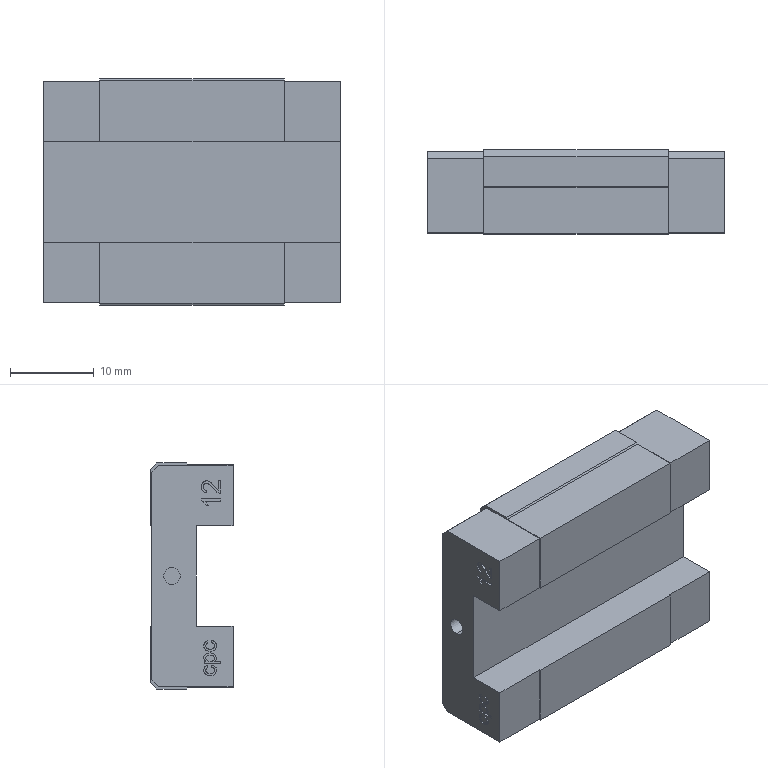Part | SolidWorks | features ICE 49, Chamfer 34, HoleWzd 16, RevCut 4, BaseBody 1 | 1 solid | 200 faces | box 35.4 x 10 x 27 mm | volume 7144 mm3 | plane 94 | spline 70 | cylinder 20 | cone 16 | commonest cylinder face diameters 2.5 x8 3 x8 2 x4